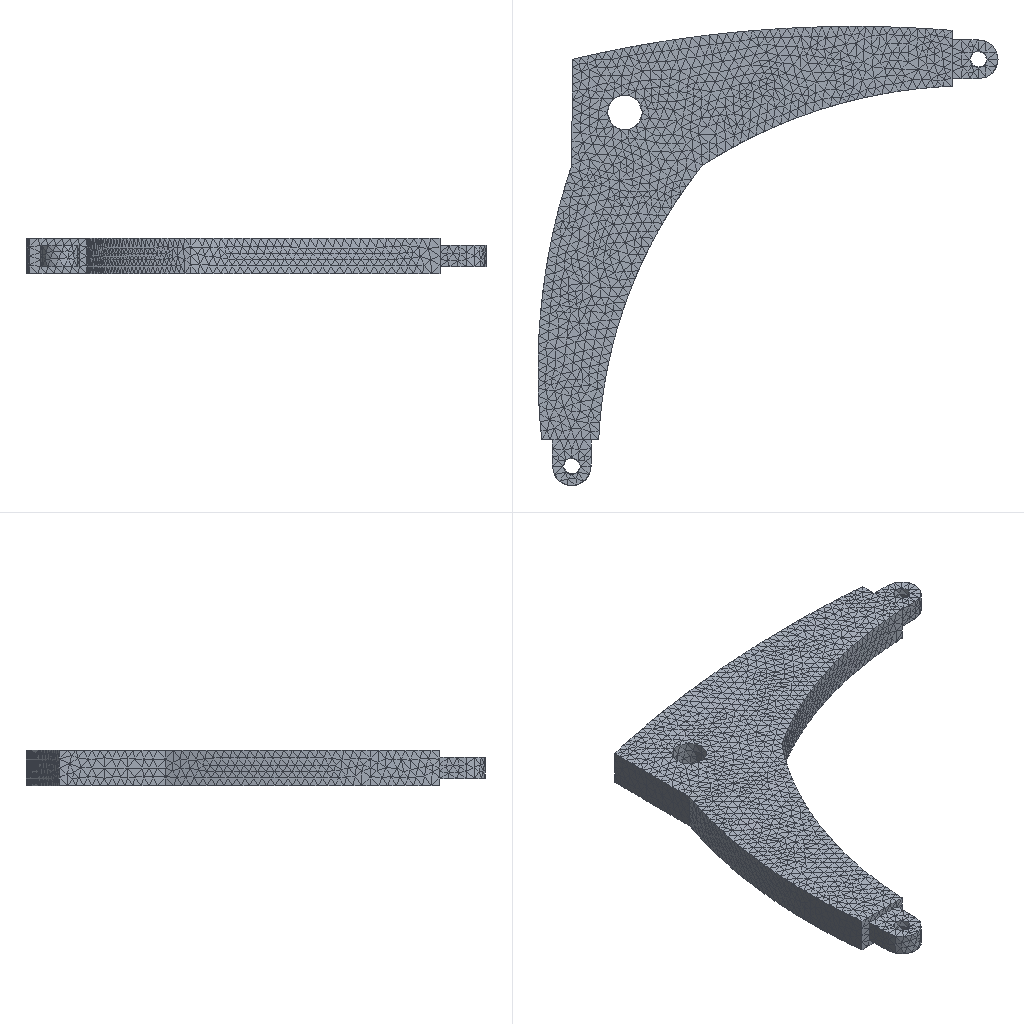Simulation study | ansys workbench
Set-up summary:
category,name,step,type,value,unit,region
solver,ansys_mapdl
solver,version,,,24.2
units,MPA,,stated
analysis,deck1
load_step,requested
analysis,nlgeom,,,False
mesh,nodes,,,0
mesh,elements,,,0
load,load commands in deck,,count,0
bc,support commands in deck,,count,0
analysis,deck2
load_step,requested
analysis,nlgeom,,,False
mesh,nodes,,,0
mesh,elements,,,0
load,load commands in deck,,count,0
bc,support commands in deck,,count,0
analysis,deck3,,static,static
load_step,requested,,,1
analysis,nlgeom,,,False
mesh,nodes,,,43385
mesh,elements,,,28503
element_type,ANSYS 187 (type 1),,solid,28414
element_type,ANSYS 174 (type 2),,contact,44
element_type,ANSYS 170 (type 3),,target,0
element_type,ANSYS 14 (type 4),,spring,1
element_type,ANSYS 154 (type 5),,surface,44
load,load commands in deck,,count,3
bc,support commands in deck,,count,3
named_set,ALLGROUNDEDSPRINGS,,component
named_set,_ELMISC,,component
named_set,_FRICSUX,,component
named_set,_FRICSUZ,,component
material,1,,in results
check,setup vs results,,match,"results also hold 0 node(s) and 1 element(s) the deck makes with ['EN']; those were not compared; 1 setup node(s) no element uses are not in the results (e.g. [43385]); 243 node(s) the deck places when it runs (an expression or NMODIF) were not compared by position (e.g. [160, 161, 162]); 1 node(s) the solver created internally for pilot nodes (ZST-1/廷旭-23个(1)/有限元仿真/拓扑优化2/拓扑优化2_files/dp0/SYS/MECH/solve.out) are in the results only; 44 surface effect element(s) are not in the reader's mesh and were not compared"
Results summary:
result,analysis,,,static
result,last_loadstep,,,1
result,primary field,,,displacement
result,reaction total,1,FX,-1499.664,N
result,reaction total,1,FY,-1499.664,N
result,reaction total,1,FZ,-3e-06,N
result,mass,,,0.000197,"NMM: mm, ton, N, s, mV, mA, degC"